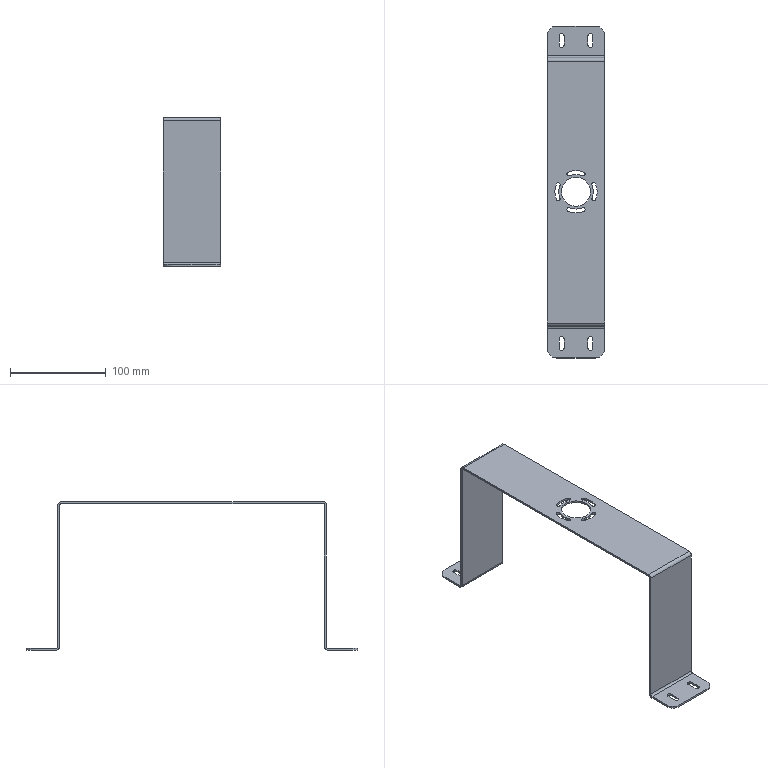Part | SolidWorks | features EdgeFlange 4, SMBaseFlange 2, Fillet 1, FlatPattern 1, ICE 1, MirrorPattern 1, SheetMetal 1 | 1 solid | 82 faces | box 60 x 346 x 155 mm | volume 74881 mm3 | cylinder 44 | plane 38 | commonest cylinder face diameters 4 x15 5 x8 36 x5 44 x5 20 x4 8 x3